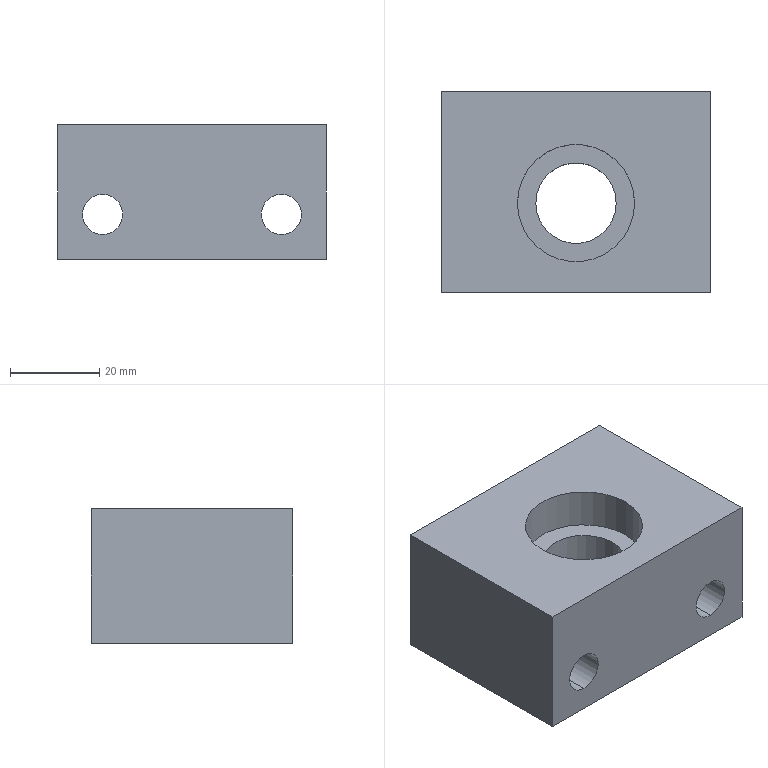Part | SolidWorks | features ICE 2, Extrusion 1, HoleWzd 1 | 1 solid | 24 faces | box 60 x 45 x 30 mm | volume 60481 mm3 | cylinder 14 | plane 10 | commonest cylinder face diameters 9 x4 15 x4 26.2 x4 18 x2
STEP:
#1=CARTESIAN_POINT('',(13.1,0.,9.));
#2=VERTEX_POINT('',#1);
#3=CARTESIAN_POINT('',(-13.1,0.,9.));
#4=VERTEX_POINT('',#3);
#5=CARTESIAN_POINT('',(0.,0.,9.));
#6=DIRECTION('',(0.,0.,-1.));
#7=DIRECTION('',(-1.,0.,0.));
#8=AXIS2_PLACEMENT_3D('',#5,#6,#7);
#9=CIRCLE('',#8,13.1);
#10=EDGE_CURVE('',#2,#4,#9,.T.);
#11=ORIENTED_EDGE('',*,*,#10,.F.);
#12=CARTESIAN_POINT('',(13.1,0.,0.));
#13=VERTEX_POINT('',#12);
#14=CARTESIAN_POINT('',(13.1,0.,9.));
#15=DIRECTION('',(0.,0.,-1.));
#16=VECTOR('',#15,1000.);
#17=LINE('',#14,#16);
#18=EDGE_CURVE('',#2,#13,#17,.T.);
#19=ORIENTED_EDGE('',*,*,#18,.T.);
#20=CARTESIAN_POINT('',(-13.1,0.,0.));
#21=VERTEX_POINT('',#20);
#22=CARTESIAN_POINT('',(0.,0.,0.));
#23=DIRECTION('',(0.,0.,-1.));
#24=DIRECTION('',(-1.,0.,0.));
#25=AXIS2_PLACEMENT_3D('',#22,#23,#24);
#26=CIRCLE('',#25,13.1);
#27=EDGE_CURVE('',#13,#21,#26,.T.);
#28=ORIENTED_EDGE('',*,*,#27,.T.);
#29=CARTESIAN_POINT('',(-13.1,0.,9.));
#30=DIRECTION('',(0.,0.,-1.));
#31=VECTOR('',#30,1000.);
#32=LINE('',#29,#31);
#33=EDGE_CURVE('',#4,#21,#32,.T.);
#34=ORIENTED_EDGE('',*,*,#33,.F.);
#35=EDGE_LOOP('',(#11,#19,#28,#34));
#36=FACE_OUTER_BOUND('',#35,.T.);
#37=CARTESIAN_POINT('',(0.,0.,9.));
#38=DIRECTION('',(0.,0.,-1.));
#39=DIRECTION('',(-1.,0.,0.));
#40=AXIS2_PLACEMENT_3D('',#37,#38,#39);
#41=CYLINDRICAL_SURFACE('',#40,13.1);
#42=ADVANCED_FACE('',(#36),#41,.F.);
#43=CARTESIAN_POINT('',(-13.1,0.,21.));
#44=VERTEX_POINT('',#43);
#45=CARTESIAN_POINT('',(13.1,0.,21.));
#46=VERTEX_POINT('',#45);
#47=CARTESIAN_POINT('',(0.,0.,21.));
#48=DIRECTION('',(0.,0.,1.));
#49=DIRECTION('',(1.,0.,0.));
#50=AXIS2_PLACEMENT_3D('',#47,#48,#49);
#51=CIRCLE('',#50,13.1);
#52=EDGE_CURVE('',#44,#46,#51,.T.);
#53=ORIENTED_EDGE('',*,*,#52,.F.);
#54=CARTESIAN_POINT('',(-13.1,0.,30.));
#55=VERTEX_POINT('',#54);
#56=CARTESIAN_POINT('',(-13.1,0.,21.));
#57=DIRECTION('',(0.,0.,1.));
#58=VECTOR('',#57,1000.);
#59=LINE('',#56,#58);
#60=EDGE_CURVE('',#44,#55,#59,.T.);
#61=ORIENTED_EDGE('',*,*,#60,.T.);
#62=CARTESIAN_POINT('',(13.1,0.,30.));
#63=VERTEX_POINT('',#62);
#64=CARTESIAN_POINT('',(0.,0.,30.));
#65=DIRECTION('',(0.,0.,1.));
#66=DIRECTION('',(1.,0.,0.));
#67=AXIS2_PLACEMENT_3D('',#64,#65,#66);
#68=CIRCLE('',#67,13.1);
#69=EDGE_CURVE('',#55,#63,#68,.T.);
#70=ORIENTED_EDGE('',*,*,#69,.T.);
#71=CARTESIAN_POINT('',(13.1,0.,21.));
#72=DIRECTION('',(0.,0.,1.));
#73=VECTOR('',#72,1000.);
#74=LINE('',#71,#73);
#75=EDGE_CURVE('',#46,#63,#74,.T.);
#76=ORIENTED_EDGE('',*,*,#75,.F.);
#77=EDGE_LOOP('',(#53,#61,#70,#76));
#78=FACE_OUTER_BOUND('',#77,.T.);
#79=CARTESIAN_POINT('',(0.,0.,21.));
#80=DIRECTION('',(0.,0.,1.));
#81=DIRECTION('',(1.,0.,0.));
#82=AXIS2_PLACEMENT_3D('',#79,#80,#81);
#83=CYLINDRICAL_SURFACE('',#82,13.1);
#84=ADVANCED_FACE('',(#78),#83,.F.);
#85=CARTESIAN_POINT('',(-20.,16.,2.5));
#86=VERTEX_POINT('',#85);
#87=CARTESIAN_POINT('',(-20.,16.,17.5));
#88=VERTEX_POINT('',#87);
#89=CARTESIAN_POINT('',(-20.,16.,10.));
#90=DIRECTION('',(0.,1.,0.));
#91=DIRECTION('',(0.,0.,1.));
#92=AXIS2_PLACEMENT_3D('',#89,#90,#91);
#93=CIRCLE('',#92,7.5);
#94=EDGE_CURVE('',#86,#88,#93,.T.);
#95=ORIENTED_EDGE('',*,*,#94,.F.);
#96=CARTESIAN_POINT('',(-20.,25.,2.5));
#97=VERTEX_POINT('',#96);
#98=CARTESIAN_POINT('',(-20.,25.,2.5));
#99=DIRECTION('',(0.,1.,0.));
#100=VECTOR('',#99,1000.);
#101=LINE('',#98,#100);
#102=EDGE_CURVE('',#86,#97,#101,.T.);
#103=ORIENTED_EDGE('',*,*,#102,.T.);
#104=CARTESIAN_POINT('',(-20.,25.,17.5));
#105=VERTEX_POINT('',#104);
#106=CARTESIAN_POINT('',(-20.,25.,10.));
#107=DIRECTION('',(0.,1.,0.));
#108=DIRECTION('',(0.,0.,1.));
#109=AXIS2_PLACEMENT_3D('',#106,#107,#108);
#110=CIRCLE('',#109,7.5);
#111=EDGE_CURVE('',#97,#105,#110,.T.);
#112=ORIENTED_EDGE('',*,*,#111,.T.);
#113=CARTESIAN_POINT('',(-20.,25.,17.5));
#114=DIRECTION('',(0.,1.,0.));
#115=VECTOR('',#114,1000.);
#116=LINE('',#113,#115);
#117=EDGE_CURVE('',#88,#105,#116,.T.);
#118=ORIENTED_EDGE('',*,*,#117,.F.);
#119=EDGE_LOOP('',(#95,#103,#112,#118));
#120=FACE_OUTER_BOUND('',#119,.T.);
#121=CARTESIAN_POINT('',(-20.,25.,10.));
#122=DIRECTION('',(0.,1.,0.));
#123=DIRECTION('',(0.,0.,1.));
#124=AXIS2_PLACEMENT_3D('',#121,#122,#123);
#125=CYLINDRICAL_SURFACE('',#124,7.5);
#126=ADVANCED_FACE('',(#120),#125,.F.);
#127=CARTESIAN_POINT('',(-20.,-20.,5.5));
#128=VERTEX_POINT('',#127);
#129=CARTESIAN_POINT('',(-20.,-20.,14.5));
#130=VERTEX_POINT('',#129);
#131=CARTESIAN_POINT('',(-20.,-20.,10.));
#132=DIRECTION('',(0.,1.,0.));
#133=DIRECTION('',(0.,0.,1.));
#134=AXIS2_PLACEMENT_3D('',#131,#132,#133);
#135=CIRCLE('',#134,4.5);
#136=EDGE_CURVE('',#128,#130,#135,.T.);
#137=ORIENTED_EDGE('',*,*,#136,.F.);
#138=CARTESIAN_POINT('',(-20.,16.,5.5));
#139=VERTEX_POINT('',#138);
#140=CARTESIAN_POINT('',(-20.,25.,5.5));
#141=DIRECTION('',(0.,1.,0.));
#142=VECTOR('',#141,1000.);
#143=LINE('',#140,#142);
#144=EDGE_CURVE('',#128,#139,#143,.T.);
#145=ORIENTED_EDGE('',*,*,#144,.T.);
#146=CARTESIAN_POINT('',(-20.,16.,14.5));
#147=VERTEX_POINT('',#146);
#148=CARTESIAN_POINT('',(-20.,16.,10.));
#149=DIRECTION('',(0.,1.,0.));
#150=DIRECTION('',(0.,0.,1.));
#151=AXIS2_PLACEMENT_3D('',#148,#149,#150);
#152=CIRCLE('',#151,4.5);
#153=EDGE_CURVE('',#139,#147,#152,.T.);
#154=ORIENTED_EDGE('',*,*,#153,.T.);
#155=CARTESIAN_POINT('',(-20.,25.,14.5));
#156=DIRECTION('',(0.,1.,0.));
#157=VECTOR('',#156,1000.);
#158=LINE('',#155,#157);
#159=EDGE_CURVE('',#130,#147,#158,.T.);
#160=ORIENTED_EDGE('',*,*,#159,.F.);
#161=EDGE_LOOP('',(#137,#145,#154,#160));
#162=FACE_OUTER_BOUND('',#161,.T.);
#163=CARTESIAN_POINT('',(-20.,25.,10.));
#164=DIRECTION('',(0.,1.,0.));
#165=DIRECTION('',(0.,0.,1.));
#166=AXIS2_PLACEMENT_3D('',#163,#164,#165);
#167=CYLINDRICAL_SURFACE('',#166,4.5);
#168=ADVANCED_FACE('',(#162),#167,.F.);
#169=CARTESIAN_POINT('',(20.,16.,2.5));
#170=VERTEX_POINT('',#169);
#171=CARTESIAN_POINT('',(20.,16.,17.5));
#172=VERTEX_POINT('',#171);
#173=CARTESIAN_POINT('',(20.,16.,10.));
#174=DIRECTION('',(0.,1.,0.));
#175=DIRECTION('',(0.,0.,1.));
#176=AXIS2_PLACEMENT_3D('',#173,#174,#175);
#177=CIRCLE('',#176,7.5);
#178=EDGE_CURVE('',#170,#172,#177,.T.);
#179=ORIENTED_EDGE('',*,*,#178,.F.);
#180=CARTESIAN_POINT('',(20.,25.,2.5));
#181=VERTEX_POINT('',#180);
#182=CARTESIAN_POINT('',(20.,25.,2.5));
#183=DIRECTION('',(0.,1.,0.));
#184=VECTOR('',#183,1000.);
#185=LINE('',#182,#184);
#186=EDGE_CURVE('',#170,#181,#185,.T.);
#187=ORIENTED_EDGE('',*,*,#186,.T.);
#188=CARTESIAN_POINT('',(20.,25.,17.5));
#189=VERTEX_POINT('',#188);
#190=CARTESIAN_POINT('',(20.,25.,10.));
#191=DIRECTION('',(0.,1.,0.));
#192=DIRECTION('',(0.,0.,1.));
#193=AXIS2_PLACEMENT_3D('',#190,#191,#192);
#194=CIRCLE('',#193,7.5);
#195=EDGE_CURVE('',#181,#189,#194,.T.);
#196=ORIENTED_EDGE('',*,*,#195,.T.);
#197=CARTESIAN_POINT('',(20.,25.,17.5));
#198=DIRECTION('',(0.,1.,0.));
#199=VECTOR('',#198,1000.);
#200=LINE('',#197,#199);
#201=EDGE_CURVE('',#172,#189,#200,.T.);
#202=ORIENTED_EDGE('',*,*,#201,.F.);
#203=EDGE_LOOP('',(#179,#187,#196,#202));
#204=FACE_OUTER_BOUND('',#203,.T.);
#205=CARTESIAN_POINT('',(20.,25.,10.));
#206=DIRECTION('',(0.,1.,0.));
#207=DIRECTION('',(0.,0.,1.));
#208=AXIS2_PLACEMENT_3D('',#205,#206,#207);
#209=CYLINDRICAL_SURFACE('',#208,7.5);
#210=ADVANCED_FACE('',(#204),#209,.F.);
#211=CARTESIAN_POINT('',(20.,-20.,5.5));
#212=VERTEX_POINT('',#211);
#213=CARTESIAN_POINT('',(20.,-20.,14.5));
#214=VERTEX_POINT('',#213);
#215=CARTESIAN_POINT('',(20.,-20.,10.));
#216=DIRECTION('',(0.,1.,0.));
#217=DIRECTION('',(0.,0.,1.));
#218=AXIS2_PLACEMENT_3D('',#215,#216,#217);
#219=CIRCLE('',#218,4.5);
#220=EDGE_CURVE('',#212,#214,#219,.T.);
#221=ORIENTED_EDGE('',*,*,#220,.F.);
#222=CARTESIAN_POINT('',(20.,16.,5.5));
#223=VERTEX_POINT('',#222);
#224=CARTESIAN_POINT('',(20.,25.,5.5));
#225=DIRECTION('',(0.,1.,0.));
#226=VECTOR('',#225,1000.);
#227=LINE('',#224,#226);
#228=EDGE_CURVE('',#212,#223,#227,.T.);
#229=ORIENTED_EDGE('',*,*,#228,.T.);
#230=CARTESIAN_POINT('',(20.,16.,14.5));
#231=VERTEX_POINT('',#230);
#232=CARTESIAN_POINT('',(20.,16.,10.));
#233=DIRECTION('',(0.,1.,0.));
#234=DIRECTION('',(0.,0.,1.));
#235=AXIS2_PLACEMENT_3D('',#232,#233,#234);
#236=CIRCLE('',#235,4.5);
#237=EDGE_CURVE('',#223,#231,#236,.T.);
#238=ORIENTED_EDGE('',*,*,#237,.T.);
#239=CARTESIAN_POINT('',(20.,25.,14.5));
#240=DIRECTION('',(0.,1.,0.));
#241=VECTOR('',#240,1000.);
#242=LINE('',#239,#241);
#243=EDGE_CURVE('',#214,#231,#242,.T.);
#244=ORIENTED_EDGE('',*,*,#243,.F.);
#245=EDGE_LOOP('',(#221,#229,#238,#244));
#246=FACE_OUTER_BOUND('',#245,.T.);
#247=CARTESIAN_POINT('',(20.,25.,10.));
#248=DIRECTION('',(0.,1.,0.));
#249=DIRECTION('',(0.,0.,1.));
#250=AXIS2_PLACEMENT_3D('',#247,#248,#249);
#251=CYLINDRICAL_SURFACE('',#250,4.5);
#252=ADVANCED_FACE('',(#246),#251,.F.);
#253=CARTESIAN_POINT('',(-9.,0.,21.));
#254=VERTEX_POINT('',#253);
#255=CARTESIAN_POINT('',(9.,0.,21.));
#256=VERTEX_POINT('',#255);
#257=CARTESIAN_POINT('',(0.,0.,21.));
#258=DIRECTION('',(0.,0.,1.));
#259=DIRECTION('',(1.,0.,0.));
#260=AXIS2_PLACEMENT_3D('',#257,#258,#259);
#261=CIRCLE('',#260,9.);
#262=EDGE_CURVE('',#254,#256,#261,.T.);
#263=ORIENTED_EDGE('',*,*,#262,.T.);
#264=CARTESIAN_POINT('',(9.,0.,9.));
#265=VERTEX_POINT('',#264);
#266=CARTESIAN_POINT('',(9.,0.,30.));
#267=DIRECTION('',(0.,0.,-1.));
#268=VECTOR('',#267,1000.);
#269=LINE('',#266,#268);
#270=EDGE_CURVE('',#256,#265,#269,.T.);
#271=ORIENTED_EDGE('',*,*,#270,.T.);
#272=CARTESIAN_POINT('',(-9.,0.,9.));
#273=VERTEX_POINT('',#272);
#274=CARTESIAN_POINT('',(0.,0.,9.));
#275=DIRECTION('',(0.,0.,-1.));
#276=DIRECTION('',(-1.,0.,0.));
#277=AXIS2_PLACEMENT_3D('',#274,#275,#276);
#278=CIRCLE('',#277,9.);
#279=EDGE_CURVE('',#265,#273,#278,.T.);
#280=ORIENTED_EDGE('',*,*,#279,.T.);
#281=CARTESIAN_POINT('',(-9.,0.,30.));
#282=DIRECTION('',(0.,0.,-1.));
#283=VECTOR('',#282,1000.);
#284=LINE('',#281,#283);
#285=EDGE_CURVE('',#254,#273,#284,.T.);
#286=ORIENTED_EDGE('',*,*,#285,.F.);
#287=EDGE_LOOP('',(#263,#271,#280,#286));
#288=FACE_OUTER_BOUND('',#287,.T.);
#289=CARTESIAN_POINT('',(0.,0.,30.));
#290=DIRECTION('',(0.,0.,-1.));
#291=DIRECTION('',(-1.,0.,0.));
#292=AXIS2_PLACEMENT_3D('',#289,#290,#291);
#293=CYLINDRICAL_SURFACE('',#292,9.);
#294=ADVANCED_FACE('',(#288),#293,.F.);
#295=ORIENTED_EDGE('',*,*,#270,.F.);
#296=CARTESIAN_POINT('',(0.,0.,21.));
#297=DIRECTION('',(0.,0.,1.));
#298=DIRECTION('',(1.,0.,0.));
#299=AXIS2_PLACEMENT_3D('',#296,#297,#298);
#300=CIRCLE('',#299,9.);
#301=EDGE_CURVE('',#256,#254,#300,.T.);
#302=ORIENTED_EDGE('',*,*,#301,.T.);
#303=ORIENTED_EDGE('',*,*,#285,.T.);
#304=CARTESIAN_POINT('',(0.,0.,9.));
#305=DIRECTION('',(0.,0.,-1.));
#306=DIRECTION('',(-1.,0.,0.));
#307=AXIS2_PLACEMENT_3D('',#304,#305,#306);
#308=CIRCLE('',#307,9.);
#309=EDGE_CURVE('',#273,#265,#308,.T.);
#310=ORIENTED_EDGE('',*,*,#309,.T.);
#311=EDGE_LOOP('',(#295,#302,#303,#310));
#312=FACE_OUTER_BOUND('',#311,.T.);
#313=CARTESIAN_POINT('',(0.,0.,30.));
#314=DIRECTION('',(0.,0.,-1.));
#315=DIRECTION('',(-1.,0.,0.));
#316=AXIS2_PLACEMENT_3D('',#313,#314,#315);
#317=CYLINDRICAL_SURFACE('',#316,9.);
#318=ADVANCED_FACE('',(#312),#317,.F.);
#319=CARTESIAN_POINT('',(0.,0.,30.));
#320=DIRECTION('',(0.,0.,1.));
#321=DIRECTION('',(1.,0.,0.));
#322=AXIS2_PLACEMENT_3D('',#319,#320,#321);
#323=CIRCLE('',#322,13.1);
#324=EDGE_CURVE('',#63,#55,#323,.T.);
#325=ORIENTED_EDGE('',*,*,#324,.F.);
#326=ORIENTED_EDGE('',*,*,#69,.F.);
#327=EDGE_LOOP('',(#325,#326));
#328=FACE_BOUND('',#327,.T.);
#329=CARTESIAN_POINT('',(-30.,25.,30.));
#330=VERTEX_POINT('',#329);
#331=CARTESIAN_POINT('',(-30.,-20.,30.));
#332=VERTEX_POINT('',#331);
#333=CARTESIAN_POINT('',(-30.,-20.,30.));
#334=DIRECTION('',(0.,-1.,0.));
#335=VECTOR('',#334,1000.);
#336=LINE('',#333,#335);
#337=EDGE_CURVE('',#330,#332,#336,.T.);
#338=ORIENTED_EDGE('',*,*,#337,.T.);
#339=CARTESIAN_POINT('',(30.,-20.,30.));
#340=VERTEX_POINT('',#339);
#341=CARTESIAN_POINT('',(-30.,-20.,30.));
#342=DIRECTION('',(1.,0.,0.));
#343=VECTOR('',#342,1000.);
#344=LINE('',#341,#343);
#345=EDGE_CURVE('',#332,#340,#344,.T.);
#346=ORIENTED_EDGE('',*,*,#345,.T.);
#347=CARTESIAN_POINT('',(30.,25.,30.));
#348=VERTEX_POINT('',#347);
#349=CARTESIAN_POINT('',(30.,-20.,30.));
#350=DIRECTION('',(0.,1.,0.));
#351=VECTOR('',#350,1000.);
#352=LINE('',#349,#351);
#353=EDGE_CURVE('',#340,#348,#352,.T.);
#354=ORIENTED_EDGE('',*,*,#353,.T.);
#355=CARTESIAN_POINT('',(-30.,25.,30.));
#356=DIRECTION('',(-1.,0.,0.));
#357=VECTOR('',#356,1000.);
#358=LINE('',#355,#357);
#359=EDGE_CURVE('',#348,#330,#358,.T.);
#360=ORIENTED_EDGE('',*,*,#359,.T.);
#361=EDGE_LOOP('',(#338,#346,#354,#360));
#362=FACE_OUTER_BOUND('',#361,.T.);
#363=CARTESIAN_POINT('',(-30.,25.,30.));
#364=DIRECTION('',(0.,0.,-1.));
#365=DIRECTION('',(-1.,0.,0.));
#366=AXIS2_PLACEMENT_3D('',#363,#364,#365);
#367=PLANE('',#366);
#368=ADVANCED_FACE('',(#328,#362),#367,.F.);
#369=CARTESIAN_POINT('',(0.,0.,0.));
#370=DIRECTION('',(0.,0.,-1.));
#371=DIRECTION('',(-1.,0.,0.));
#372=AXIS2_PLACEMENT_3D('',#369,#370,#371);
#373=CIRCLE('',#372,13.1);
#374=EDGE_CURVE('',#21,#13,#373,.T.);
#375=ORIENTED_EDGE('',*,*,#374,.F.);
#376=ORIENTED_EDGE('',*,*,#27,.F.);
#377=EDGE_LOOP('',(#375,#376));
#378=FACE_BOUND('',#377,.T.);
#379=CARTESIAN_POINT('',(-30.,25.,0.));
#380=VERTEX_POINT('',#379);
#381=CARTESIAN_POINT('',(-30.,-20.,0.));
#382=VERTEX_POINT('',#381);
#383=CARTESIAN_POINT('',(-30.,-20.,0.));
#384=DIRECTION('',(0.,-1.,0.));
#385=VECTOR('',#384,1000.);
#386=LINE('',#383,#385);
#387=EDGE_CURVE('',#380,#382,#386,.T.);
#388=ORIENTED_EDGE('',*,*,#387,.F.);
#389=CARTESIAN_POINT('',(30.,25.,0.));
#390=VERTEX_POINT('',#389);
#391=CARTESIAN_POINT('',(-30.,25.,0.));
#392=DIRECTION('',(-1.,0.,0.));
#393=VECTOR('',#392,1000.);
#394=LINE('',#391,#393);
#395=EDGE_CURVE('',#390,#380,#394,.T.);
#396=ORIENTED_EDGE('',*,*,#395,.F.);
#397=CARTESIAN_POINT('',(30.,-20.,0.));
#398=VERTEX_POINT('',#397);
#399=CARTESIAN_POINT('',(30.,-20.,0.));
#400=DIRECTION('',(0.,1.,0.));
#401=VECTOR('',#400,1000.);
#402=LINE('',#399,#401);
#403=EDGE_CURVE('',#398,#390,#402,.T.);
#404=ORIENTED_EDGE('',*,*,#403,.F.);
#405=CARTESIAN_POINT('',(-30.,-20.,0.));
#406=DIRECTION('',(1.,0.,0.));
#407=VECTOR('',#406,1000.);
#408=LINE('',#405,#407);
#409=EDGE_CURVE('',#382,#398,#408,.T.);
#410=ORIENTED_EDGE('',*,*,#409,.F.);
#411=EDGE_LOOP('',(#388,#396,#404,#410));
#412=FACE_OUTER_BOUND('',#411,.T.);
#413=CARTESIAN_POINT('',(-30.,25.,0.));
#414=DIRECTION('',(0.,0.,-1.));
#415=DIRECTION('',(-1.,0.,0.));
#416=AXIS2_PLACEMENT_3D('',#413,#414,#415);
#417=PLANE('',#416);
#418=ADVANCED_FACE('',(#378,#412),#417,.T.);
#419=ORIENTED_EDGE('',*,*,#387,.T.);
#420=CARTESIAN_POINT('',(-30.,-20.,30.));
#421=DIRECTION('',(0.,0.,-1.));
#422=VECTOR('',#421,1000.);
#423=LINE('',#420,#422);
#424=EDGE_CURVE('',#332,#382,#423,.T.);
#425=ORIENTED_EDGE('',*,*,#424,.F.);
#426=ORIENTED_EDGE('',*,*,#337,.F.);
#427=CARTESIAN_POINT('',(-30.,25.,30.));
#428=DIRECTION('',(0.,0.,-1.));
#429=VECTOR('',#428,1000.);
#430=LINE('',#427,#429);
#431=EDGE_CURVE('',#330,#380,#430,.T.);
#432=ORIENTED_EDGE('',*,*,#431,.T.);
#433=EDGE_LOOP('',(#419,#425,#426,#432));
#434=FACE_OUTER_BOUND('',#433,.T.);
#435=CARTESIAN_POINT('',(-30.,-20.,30.));
#436=DIRECTION('',(1.,0.,0.));
#437=DIRECTION('',(0.,0.,-1.));
#438=AXIS2_PLACEMENT_3D('',#435,#436,#437);
#439=PLANE('',#438);
#440=ADVANCED_FACE('',(#434),#439,.F.);
#441=CARTESIAN_POINT('',(-20.,-20.,10.));
#442=DIRECTION('',(0.,1.,0.));
#443=DIRECTION('',(0.,0.,1.));
#444=AXIS2_PLACEMENT_3D('',#441,#442,#443);
#445=CIRCLE('',#444,4.5);
#446=EDGE_CURVE('',#130,#128,#445,.T.);
#447=ORIENTED_EDGE('',*,*,#446,.T.);
#448=ORIENTED_EDGE('',*,*,#136,.T.);
#449=EDGE_LOOP('',(#447,#448));
#450=FACE_BOUND('',#449,.T.);
#451=CARTESIAN_POINT('',(20.,-20.,10.));
#452=DIRECTION('',(0.,1.,0.));
#453=DIRECTION('',(0.,0.,1.));
#454=AXIS2_PLACEMENT_3D('',#451,#452,#453);
#455=CIRCLE('',#454,4.5);
#456=EDGE_CURVE('',#214,#212,#455,.T.);
#457=ORIENTED_EDGE('',*,*,#456,.T.);
#458=ORIENTED_EDGE('',*,*,#220,.T.);
#459=EDGE_LOOP('',(#457,#458));
#460=FACE_BOUND('',#459,.T.);
#461=ORIENTED_EDGE('',*,*,#409,.T.);
#462=CARTESIAN_POINT('',(30.,-20.,30.));
#463=DIRECTION('',(0.,0.,-1.));
#464=VECTOR('',#463,1000.);
#465=LINE('',#462,#464);
#466=EDGE_CURVE('',#340,#398,#465,.T.);
#467=ORIENTED_EDGE('',*,*,#466,.F.);
#468=ORIENTED_EDGE('',*,*,#345,.F.);
#469=ORIENTED_EDGE('',*,*,#424,.T.);
#470=EDGE_LOOP('',(#461,#467,#468,#469));
#471=FACE_OUTER_BOUND('',#470,.T.);
#472=CARTESIAN_POINT('',(-30.,-20.,30.));
#473=DIRECTION('',(0.,1.,0.));
#474=DIRECTION('',(0.,0.,1.));
#475=AXIS2_PLACEMENT_3D('',#472,#473,#474);
#476=PLANE('',#475);
#477=ADVANCED_FACE('',(#450,#460,#471),#476,.F.);
#478=ORIENTED_EDGE('',*,*,#403,.T.);
#479=CARTESIAN_POINT('',(30.,25.,30.));
#480=DIRECTION('',(0.,0.,-1.));
#481=VECTOR('',#480,1000.);
#482=LINE('',#479,#481);
#483=EDGE_CURVE('',#348,#390,#482,.T.);
#484=ORIENTED_EDGE('',*,*,#483,.F.);
#485=ORIENTED_EDGE('',*,*,#353,.F.);
#486=ORIENTED_EDGE('',*,*,#466,.T.);
#487=EDGE_LOOP('',(#478,#484,#485,#486));
#488=FACE_OUTER_BOUND('',#487,.T.);
#489=CARTESIAN_POINT('',(30.,-20.,30.));
#490=DIRECTION('',(-1.,0.,0.));
#491=DIRECTION('',(0.,0.,1.));
#492=AXIS2_PLACEMENT_3D('',#489,#490,#491);
#493=PLANE('',#492);
#494=ADVANCED_FACE('',(#488),#493,.F.);
#495=CARTESIAN_POINT('',(-20.,25.,10.));
#496=DIRECTION('',(0.,1.,0.));
#497=DIRECTION('',(0.,0.,1.));
#498=AXIS2_PLACEMENT_3D('',#495,#496,#497);
#499=CIRCLE('',#498,7.5);
#500=EDGE_CURVE('',#105,#97,#499,.T.);
#501=ORIENTED_EDGE('',*,*,#500,.F.);
#502=ORIENTED_EDGE('',*,*,#111,.F.);
#503=EDGE_LOOP('',(#501,#502));
#504=FACE_BOUND('',#503,.T.);
#505=CARTESIAN_POINT('',(20.,25.,10.));
#506=DIRECTION('',(0.,1.,0.));
#507=DIRECTION('',(0.,0.,1.));
#508=AXIS2_PLACEMENT_3D('',#505,#506,#507);
#509=CIRCLE('',#508,7.5);
#510=EDGE_CURVE('',#189,#181,#509,.T.);
#511=ORIENTED_EDGE('',*,*,#510,.F.);
#512=ORIENTED_EDGE('',*,*,#195,.F.);
#513=EDGE_LOOP('',(#511,#512));
#514=FACE_BOUND('',#513,.T.);
#515=ORIENTED_EDGE('',*,*,#395,.T.);
#516=ORIENTED_EDGE('',*,*,#431,.F.);
#517=ORIENTED_EDGE('',*,*,#359,.F.);
#518=ORIENTED_EDGE('',*,*,#483,.T.);
#519=EDGE_LOOP('',(#515,#516,#517,#518));
#520=FACE_OUTER_BOUND('',#519,.T.);
#521=CARTESIAN_POINT('',(-30.,25.,30.));
#522=DIRECTION('',(0.,-1.,0.));
#523=DIRECTION('',(0.,0.,-1.));
#524=AXIS2_PLACEMENT_3D('',#521,#522,#523);
#525=PLANE('',#524);
#526=ADVANCED_FACE('',(#504,#514,#520),#525,.F.);
#527=ORIENTED_EDGE('',*,*,#228,.F.);
#528=ORIENTED_EDGE('',*,*,#456,.F.);
#529=ORIENTED_EDGE('',*,*,#243,.T.);
#530=CARTESIAN_POINT('',(20.,16.,10.));
#531=DIRECTION('',(0.,1.,0.));
#532=DIRECTION('',(0.,0.,1.));
#533=AXIS2_PLACEMENT_3D('',#530,#531,#532);
#534=CIRCLE('',#533,4.5);
#535=EDGE_CURVE('',#231,#223,#534,.T.);
#536=ORIENTED_EDGE('',*,*,#535,.T.);
#537=EDGE_LOOP('',(#527,#528,#529,#536));
#538=FACE_OUTER_BOUND('',#537,.T.);
#539=CARTESIAN_POINT('',(20.,25.,10.));
#540=DIRECTION('',(0.,1.,0.));
#541=DIRECTION('',(0.,0.,1.));
#542=AXIS2_PLACEMENT_3D('',#539,#540,#541);
#543=CYLINDRICAL_SURFACE('',#542,4.5);
#544=ADVANCED_FACE('',(#538),#543,.F.);
#545=ORIENTED_EDGE('',*,*,#535,.F.);
#546=ORIENTED_EDGE('',*,*,#237,.F.);
#547=EDGE_LOOP('',(#545,#546));
#548=FACE_BOUND('',#547,.T.);
#549=CARTESIAN_POINT('',(20.,16.,10.));
#550=DIRECTION('',(0.,1.,0.));
#551=DIRECTION('',(0.,0.,1.));
#552=AXIS2_PLACEMENT_3D('',#549,#550,#551);
#553=CIRCLE('',#552,7.5);
#554=EDGE_CURVE('',#172,#170,#553,.T.);
#555=ORIENTED_EDGE('',*,*,#554,.T.);
#556=ORIENTED_EDGE('',*,*,#178,.T.);
#557=EDGE_LOOP('',(#555,#556));
#558=FACE_OUTER_BOUND('',#557,.T.);
#559=CARTESIAN_POINT('',(24.5,16.,10.));
#560=DIRECTION('',(0.,-1.,0.));
#561=DIRECTION('',(0.,0.,-1.));
#562=AXIS2_PLACEMENT_3D('',#559,#560,#561);
#563=PLANE('',#562);
#564=ADVANCED_FACE('',(#548,#558),#563,.F.);
#565=ORIENTED_EDGE('',*,*,#186,.F.);
#566=ORIENTED_EDGE('',*,*,#554,.F.);
#567=ORIENTED_EDGE('',*,*,#201,.T.);
#568=ORIENTED_EDGE('',*,*,#510,.T.);
#569=EDGE_LOOP('',(#565,#566,#567,#568));
#570=FACE_OUTER_BOUND('',#569,.T.);
#571=CARTESIAN_POINT('',(20.,25.,10.));
#572=DIRECTION('',(0.,1.,0.));
#573=DIRECTION('',(0.,0.,1.));
#574=AXIS2_PLACEMENT_3D('',#571,#572,#573);
#575=CYLINDRICAL_SURFACE('',#574,7.5);
#576=ADVANCED_FACE('',(#570),#575,.F.);
#577=ORIENTED_EDGE('',*,*,#144,.F.);
#578=ORIENTED_EDGE('',*,*,#446,.F.);
#579=ORIENTED_EDGE('',*,*,#159,.T.);
#580=CARTESIAN_POINT('',(-20.,16.,10.));
#581=DIRECTION('',(0.,1.,0.));
#582=DIRECTION('',(0.,0.,1.));
#583=AXIS2_PLACEMENT_3D('',#580,#581,#582);
#584=CIRCLE('',#583,4.5);
#585=EDGE_CURVE('',#147,#139,#584,.T.);
#586=ORIENTED_EDGE('',*,*,#585,.T.);
#587=EDGE_LOOP('',(#577,#578,#579,#586));
#588=FACE_OUTER_BOUND('',#587,.T.);
#589=CARTESIAN_POINT('',(-20.,25.,10.));
#590=DIRECTION('',(0.,1.,0.));
#591=DIRECTION('',(0.,0.,1.));
#592=AXIS2_PLACEMENT_3D('',#589,#590,#591);
#593=CYLINDRICAL_SURFACE('',#592,4.5);
#594=ADVANCED_FACE('',(#588),#593,.F.);
#595=ORIENTED_EDGE('',*,*,#585,.F.);
#596=ORIENTED_EDGE('',*,*,#153,.F.);
#597=EDGE_LOOP('',(#595,#596));
#598=FACE_BOUND('',#597,.T.);
#599=CARTESIAN_POINT('',(-20.,16.,10.));
#600=DIRECTION('',(0.,1.,0.));
#601=DIRECTION('',(0.,0.,1.));
#602=AXIS2_PLACEMENT_3D('',#599,#600,#601);
#603=CIRCLE('',#602,7.5);
#604=EDGE_CURVE('',#88,#86,#603,.T.);
#605=ORIENTED_EDGE('',*,*,#604,.T.);
#606=ORIENTED_EDGE('',*,*,#94,.T.);
#607=EDGE_LOOP('',(#605,#606));
#608=FACE_OUTER_BOUND('',#607,.T.);
#609=CARTESIAN_POINT('',(-15.5,16.,10.));
#610=DIRECTION('',(0.,-1.,0.));
#611=DIRECTION('',(0.,0.,-1.));
#612=AXIS2_PLACEMENT_3D('',#609,#610,#611);
#613=PLANE('',#612);
#614=ADVANCED_FACE('',(#598,#608),#613,.F.);
#615=ORIENTED_EDGE('',*,*,#102,.F.);
#616=ORIENTED_EDGE('',*,*,#604,.F.);
#617=ORIENTED_EDGE('',*,*,#117,.T.);
#618=ORIENTED_EDGE('',*,*,#500,.T.);
#619=EDGE_LOOP('',(#615,#616,#617,#618));
#620=FACE_OUTER_BOUND('',#619,.T.);
#621=CARTESIAN_POINT('',(-20.,25.,10.));
#622=DIRECTION('',(0.,1.,0.));
#623=DIRECTION('',(0.,0.,1.));
#624=AXIS2_PLACEMENT_3D('',#621,#622,#623);
#625=CYLINDRICAL_SURFACE('',#624,7.5);
#626=ADVANCED_FACE('',(#620),#625,.F.);
#627=ORIENTED_EDGE('',*,*,#60,.F.);
#628=CARTESIAN_POINT('',(0.,0.,21.));
#629=DIRECTION('',(0.,0.,1.));
#630=DIRECTION('',(1.,0.,0.));
#631=AXIS2_PLACEMENT_3D('',#628,#629,#630);
#632=CIRCLE('',#631,13.1);
#633=EDGE_CURVE('',#46,#44,#632,.T.);
#634=ORIENTED_EDGE('',*,*,#633,.F.);
#635=ORIENTED_EDGE('',*,*,#75,.T.);
#636=ORIENTED_EDGE('',*,*,#324,.T.);
#637=EDGE_LOOP('',(#627,#634,#635,#636));
#638=FACE_OUTER_BOUND('',#637,.T.);
#639=CARTESIAN_POINT('',(0.,0.,21.));
#640=DIRECTION('',(0.,0.,1.));
#641=DIRECTION('',(1.,0.,0.));
#642=AXIS2_PLACEMENT_3D('',#639,#640,#641);
#643=CYLINDRICAL_SURFACE('',#642,13.1);
#644=ADVANCED_FACE('',(#638),#643,.F.);
#645=ORIENTED_EDGE('',*,*,#262,.F.);
#646=ORIENTED_EDGE('',*,*,#301,.F.);
#647=EDGE_LOOP('',(#645,#646));
#648=FACE_BOUND('',#647,.T.);
#649=ORIENTED_EDGE('',*,*,#633,.T.);
#650=ORIENTED_EDGE('',*,*,#52,.T.);
#651=EDGE_LOOP('',(#649,#650));
#652=FACE_OUTER_BOUND('',#651,.T.);
#653=CARTESIAN_POINT('',(0.,0.,21.));
#654=DIRECTION('',(0.,0.,1.));
#655=DIRECTION('',(1.,0.,0.));
#656=AXIS2_PLACEMENT_3D('',#653,#654,#655);
#657=PLANE('',#656);
#658=ADVANCED_FACE('',(#648,#652),#657,.T.);
#659=ORIENTED_EDGE('',*,*,#18,.F.);
#660=CARTESIAN_POINT('',(0.,0.,9.));
#661=DIRECTION('',(0.,0.,-1.));
#662=DIRECTION('',(-1.,0.,0.));
#663=AXIS2_PLACEMENT_3D('',#660,#661,#662);
#664=CIRCLE('',#663,13.1);
#665=EDGE_CURVE('',#4,#2,#664,.T.);
#666=ORIENTED_EDGE('',*,*,#665,.F.);
#667=ORIENTED_EDGE('',*,*,#33,.T.);
#668=ORIENTED_EDGE('',*,*,#374,.T.);
#669=EDGE_LOOP('',(#659,#666,#667,#668));
#670=FACE_OUTER_BOUND('',#669,.T.);
#671=CARTESIAN_POINT('',(0.,0.,9.));
#672=DIRECTION('',(0.,0.,-1.));
#673=DIRECTION('',(-1.,0.,0.));
#674=AXIS2_PLACEMENT_3D('',#671,#672,#673);
#675=CYLINDRICAL_SURFACE('',#674,13.1);
#676=ADVANCED_FACE('',(#670),#675,.F.);
#677=ORIENTED_EDGE('',*,*,#309,.F.);
#678=ORIENTED_EDGE('',*,*,#279,.F.);
#679=EDGE_LOOP('',(#677,#678));
#680=FACE_BOUND('',#679,.T.);
#681=ORIENTED_EDGE('',*,*,#665,.T.);
#682=ORIENTED_EDGE('',*,*,#10,.T.);
#683=EDGE_LOOP('',(#681,#682));
#684=FACE_OUTER_BOUND('',#683,.T.);
#685=CARTESIAN_POINT('',(0.,0.,9.));
#686=DIRECTION('',(0.,0.,-1.));
#687=DIRECTION('',(-1.,0.,0.));
#688=AXIS2_PLACEMENT_3D('',#685,#686,#687);
#689=PLANE('',#688);
#690=ADVANCED_FACE('',(#680,#684),#689,.T.);
#691=CLOSED_SHELL('',(#42,#84,#126,#168,#210,#252,#294,#318,#368,#418,#440,#477,#494,#526,#544,#564,#576,#594,#614,#626,#644,#658,#676,#690));
#692=MANIFOLD_SOLID_BREP('',#691);
#693=CARTESIAN_POINT('',(0.,0.,0.));
#694=DIRECTION('',(0.,0.,1.));
#695=DIRECTION('',(1.,0.,0.));
#696=AXIS2_PLACEMENT_3D('',#693,#694,#695);
#697=(LENGTH_UNIT()NAMED_UNIT(*)SI_UNIT(.MILLI.,.METRE.));
#698=UNCERTAINTY_MEASURE_WITH_UNIT(LENGTH_MEASURE(0.00001),#697,'','');
#699=(NAMED_UNIT(*)PLANE_ANGLE_UNIT()SI_UNIT($,.RADIAN.));
#700=(NAMED_UNIT(*)SI_UNIT($,.STERADIAN.)SOLID_ANGLE_UNIT());
#701=(GEOMETRIC_REPRESENTATION_CONTEXT(3)GLOBAL_UNCERTAINTY_ASSIGNED_CONTEXT((#698))GLOBAL_UNIT_ASSIGNED_CONTEXT((#697,#699,#700))REPRESENTATION_CONTEXT('',''));
#702=ADVANCED_BREP_SHAPE_REPRESENTATION('',(#692,#696),#701);